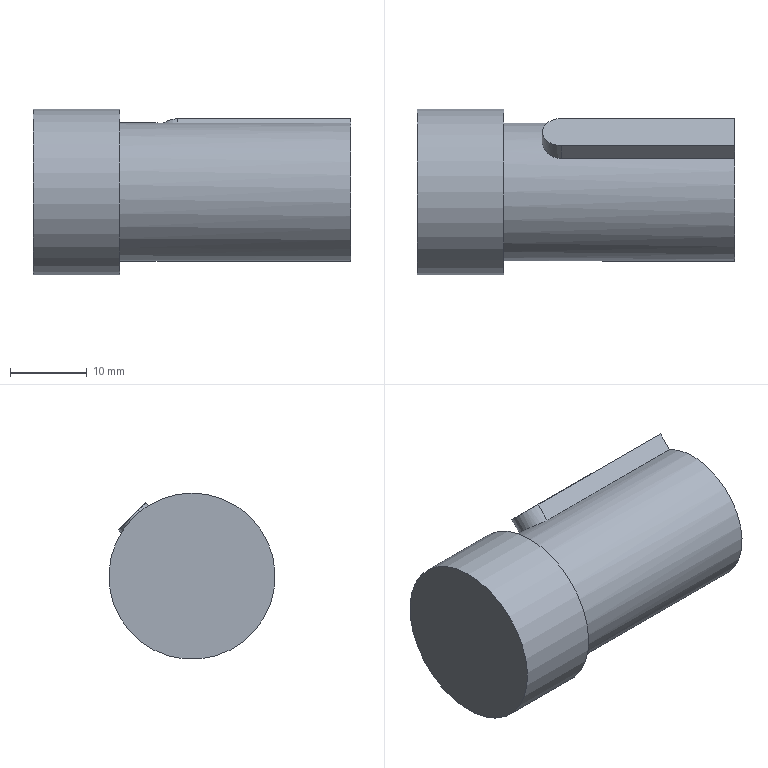Part | STEP file | basic_gh_motor_gh1_01 | 1 solid | 9 faces | box 41.25 x 21.6 x 21.6 mm | volume 12015 mm3 | plane 6 | cylinder 3 | commonest cylinder face diameters 5 x1 18 x1 21.6 x1
STEP:
#1=CARTESIAN_POINT('',(0.,92.846,7.881));
#2=VERTEX_POINT('',#1);
#3=CARTESIAN_POINT('',(-22.5,92.846,7.881));
#4=VERTEX_POINT('',#3);
#5=CARTESIAN_POINT('',(-11.25,92.846,7.881));
#6=DIRECTION('',(-1.,0.,0.));
#7=VECTOR('',#6,1.);
#8=LINE('',#5,#7);
#9=EDGE_CURVE('',#2,#4,#8,.T.);
#10=ORIENTED_EDGE('',*,*,#9,.F.);
#11=CARTESIAN_POINT('',(0.,94.51,9.546));
#12=VERTEX_POINT('',#11);
#13=CARTESIAN_POINT('',(0.,90.621,5.657));
#14=DIRECTION('',(0.,-0.7071,-0.7071));
#15=VECTOR('',#14,1.);
#16=LINE('',#13,#15);
#17=EDGE_CURVE('',#12,#2,#16,.T.);
#18=ORIENTED_EDGE('',*,*,#17,.F.);
#19=CARTESIAN_POINT('',(-22.5,94.51,9.546));
#20=VERTEX_POINT('',#19);
#21=CARTESIAN_POINT('',(-11.25,94.51,9.546));
#22=DIRECTION('',(1.,0.,0.));
#23=VECTOR('',#22,1.);
#24=LINE('',#21,#23);
#25=EDGE_CURVE('',#20,#12,#24,.T.);
#26=ORIENTED_EDGE('',*,*,#25,.F.);
#27=CARTESIAN_POINT('',(-22.5,90.621,5.657));
#28=DIRECTION('',(0.,-0.7071,-0.7071));
#29=VECTOR('',#28,1.);
#30=LINE('',#27,#29);
#31=EDGE_CURVE('',#20,#4,#30,.T.);
#32=ORIENTED_EDGE('',*,*,#31,.T.);
#33=EDGE_LOOP('',(#10,#18,#26,#32));
#34=FACE_OUTER_BOUND('',#33,.T.);
#35=CARTESIAN_POINT('',(-11.25,90.621,5.657));
#36=DIRECTION('',(0.,0.7071,-0.7071));
#37=DIRECTION('',(0.,0.7071,0.7071));
#38=AXIS2_PLACEMENT_3D('',#35,#36,#37);
#39=PLANE('',#38);
#40=ADVANCED_FACE('',(#34),#39,.F.);
#41=CARTESIAN_POINT('',(-22.5,96.381,4.346));
#42=VERTEX_POINT('',#41);
#43=CARTESIAN_POINT('',(-22.5,92.846,7.881));
#44=CARTESIAN_POINT('',(-22.658,92.846,7.881));
#45=CARTESIAN_POINT('',(-22.821,92.86,7.874));
#46=CARTESIAN_POINT('',(-23.144,92.917,7.841));
#47=CARTESIAN_POINT('',(-23.305,92.961,7.817));
#48=CARTESIAN_POINT('',(-23.613,93.076,7.75));
#49=CARTESIAN_POINT('',(-23.76,93.146,7.709));
#50=CARTESIAN_POINT('',(-24.032,93.306,7.61));
#51=CARTESIAN_POINT('',(-24.157,93.396,7.552));
#52=CARTESIAN_POINT('',(-24.378,93.584,7.428));
#53=CARTESIAN_POINT('',(-24.482,93.688,7.355));
#54=CARTESIAN_POINT('',(-24.665,93.911,7.193));
#55=CARTESIAN_POINT('',(-24.745,94.029,7.103));
#56=CARTESIAN_POINT('',(-24.873,94.27,6.909));
#57=CARTESIAN_POINT('',(-24.921,94.393,6.804));
#58=CARTESIAN_POINT('',(-24.985,94.634,6.588));
#59=CARTESIAN_POINT('',(-25.,94.752,6.476));
#60=CARTESIAN_POINT('',(-25.,94.976,6.252));
#61=CARTESIAN_POINT('',(-24.985,95.088,6.134));
#62=CARTESIAN_POINT('',(-24.921,95.304,5.893));
#63=CARTESIAN_POINT('',(-24.873,95.409,5.77));
#64=CARTESIAN_POINT('',(-24.745,95.603,5.529));
#65=CARTESIAN_POINT('',(-24.665,95.693,5.411));
#66=CARTESIAN_POINT('',(-24.482,95.855,5.188));
#67=CARTESIAN_POINT('',(-24.378,95.928,5.084));
#68=CARTESIAN_POINT('',(-24.157,96.052,4.896));
#69=CARTESIAN_POINT('',(-24.032,96.11,4.806));
#70=CARTESIAN_POINT('',(-23.76,96.209,4.646));
#71=CARTESIAN_POINT('',(-23.613,96.25,4.576));
#72=CARTESIAN_POINT('',(-23.305,96.317,4.461));
#73=CARTESIAN_POINT('',(-23.144,96.341,4.417));
#74=CARTESIAN_POINT('',(-22.821,96.374,4.36));
#75=CARTESIAN_POINT('',(-22.658,96.381,4.346));
#76=CARTESIAN_POINT('',(-22.5,96.381,4.346));
#77=B_SPLINE_CURVE_WITH_KNOTS('',3,(#43,#44,#45,#46,#47,#48,#49,#50,#51,#52,#53,#54,#55,#56,#57,#58,#59,#60,#61,#62,#63,#64,#65,#66,#67,#68,#69,#70,#71,#72,#73,#74,#75,#76),.UNSPECIFIED.,.F.,.F.,(4,2,2,2,2,2,2,2,2,2,2,2,2,2,2,2,4),(-7.577,-7.103,-6.63,-6.156,-5.682,-5.209,-4.735,-4.262,-3.788,-3.315,-2.841,-2.368,-1.894,-1.421,-0.9472,-0.4736,0.),.UNSPECIFIED.);
#78=EDGE_CURVE('',#4,#42,#77,.T.);
#79=ORIENTED_EDGE('',*,*,#78,.F.);
#80=ORIENTED_EDGE('',*,*,#31,.F.);
#81=CARTESIAN_POINT('',(-22.5,98.046,6.01));
#82=VERTEX_POINT('',#81);
#83=CARTESIAN_POINT('',(-22.5,96.278,7.778));
#84=DIRECTION('',(0.,0.7071,0.7071));
#85=DIRECTION('',(1.,0.,0.));
#86=AXIS2_PLACEMENT_3D('',#83,#84,#85);
#87=CIRCLE('',#86,2.5);
#88=EDGE_CURVE('',#82,#20,#87,.T.);
#89=ORIENTED_EDGE('',*,*,#88,.F.);
#90=CARTESIAN_POINT('',(-22.5,94.157,2.121));
#91=DIRECTION('',(0.,-0.7071,-0.7071));
#92=VECTOR('',#91,1.);
#93=LINE('',#90,#92);
#94=EDGE_CURVE('',#82,#42,#93,.T.);
#95=ORIENTED_EDGE('',*,*,#94,.T.);
#96=EDGE_LOOP('',(#79,#80,#89,#95));
#97=FACE_OUTER_BOUND('',#96,.T.);
#98=CARTESIAN_POINT('',(-22.5,92.389,3.889));
#99=DIRECTION('',(0.,0.7071,0.7071));
#100=DIRECTION('',(-1.,0.,0.));
#101=AXIS2_PLACEMENT_3D('',#98,#99,#100);
#102=CYLINDRICAL_SURFACE('',#101,2.5);
#103=ADVANCED_FACE('',(#97),#102,.T.);
#104=CARTESIAN_POINT('',(0.,98.046,6.01));
#105=VERTEX_POINT('',#104);
#106=CARTESIAN_POINT('',(-11.25,98.046,6.01));
#107=DIRECTION('',(-1.,0.,0.));
#108=VECTOR('',#107,1.);
#109=LINE('',#106,#108);
#110=EDGE_CURVE('',#105,#82,#109,.T.);
#111=ORIENTED_EDGE('',*,*,#110,.T.);
#112=ORIENTED_EDGE('',*,*,#88,.T.);
#113=ORIENTED_EDGE('',*,*,#25,.T.);
#114=CARTESIAN_POINT('',(0.,96.278,7.778));
#115=DIRECTION('',(0.,0.7071,-0.7071));
#116=VECTOR('',#115,1.);
#117=LINE('',#114,#116);
#118=EDGE_CURVE('',#12,#105,#117,.T.);
#119=ORIENTED_EDGE('',*,*,#118,.T.);
#120=EDGE_LOOP('',(#111,#112,#113,#119));
#121=FACE_OUTER_BOUND('',#120,.T.);
#122=CARTESIAN_POINT('',(-11.25,96.278,7.778));
#123=DIRECTION('',(0.,0.7071,0.7071));
#124=DIRECTION('',(1.,0.,0.));
#125=AXIS2_PLACEMENT_3D('',#122,#123,#124);
#126=PLANE('',#125);
#127=ADVANCED_FACE('',(#121),#126,.T.);
#128=CARTESIAN_POINT('',(0.,96.381,4.346));
#129=VERTEX_POINT('',#128);
#130=CARTESIAN_POINT('',(-11.25,96.381,4.346));
#131=DIRECTION('',(1.,0.,0.));
#132=VECTOR('',#131,1.);
#133=LINE('',#130,#132);
#134=EDGE_CURVE('',#42,#129,#133,.T.);
#135=ORIENTED_EDGE('',*,*,#134,.F.);
#136=ORIENTED_EDGE('',*,*,#94,.F.);
#137=ORIENTED_EDGE('',*,*,#110,.F.);
#138=CARTESIAN_POINT('',(0.,94.157,2.121));
#139=DIRECTION('',(0.,-0.7071,-0.7071));
#140=VECTOR('',#139,1.);
#141=LINE('',#138,#140);
#142=EDGE_CURVE('',#105,#129,#141,.T.);
#143=ORIENTED_EDGE('',*,*,#142,.T.);
#144=EDGE_LOOP('',(#135,#136,#137,#143));
#145=FACE_OUTER_BOUND('',#144,.T.);
#146=CARTESIAN_POINT('',(-11.25,94.157,2.121));
#147=DIRECTION('',(0.,-0.7071,0.7071));
#148=DIRECTION('',(0.,-0.7071,-0.7071));
#149=AXIS2_PLACEMENT_3D('',#146,#147,#148);
#150=PLANE('',#149);
#151=ADVANCED_FACE('',(#145),#150,.F.);
#152=CARTESIAN_POINT('',(-30.,88.5,-9.));
#153=VERTEX_POINT('',#152);
#154=CARTESIAN_POINT('',(-30.,88.5,0.));
#155=DIRECTION('',(-1.,0.,0.));
#156=DIRECTION('',(0.,0.,1.));
#157=AXIS2_PLACEMENT_3D('',#154,#155,#156);
#158=CIRCLE('',#157,9.);
#159=EDGE_CURVE('',#153,#153,#158,.T.);
#160=ORIENTED_EDGE('',*,*,#159,.F.);
#161=CARTESIAN_POINT('',(0.,88.5,-9.));
#162=VERTEX_POINT('',#161);
#163=CARTESIAN_POINT('',(-15.05,88.5,-9.));
#164=DIRECTION('',(1.,0.,0.));
#165=VECTOR('',#164,9.);
#166=LINE('',#163,#165);
#167=EDGE_CURVE('',#153,#162,#166,.T.);
#168=ORIENTED_EDGE('',*,*,#167,.T.);
#169=CARTESIAN_POINT('',(0.,88.5,0.));
#170=DIRECTION('',(1.,0.,0.));
#171=DIRECTION('',(0.,0.,1.));
#172=AXIS2_PLACEMENT_3D('',#169,#170,#171);
#173=CIRCLE('',#172,9.);
#174=EDGE_CURVE('',#2,#162,#173,.T.);
#175=ORIENTED_EDGE('',*,*,#174,.F.);
#176=ORIENTED_EDGE('',*,*,#9,.T.);
#177=ORIENTED_EDGE('',*,*,#78,.T.);
#178=ORIENTED_EDGE('',*,*,#134,.T.);
#179=CARTESIAN_POINT('',(0.,88.5,0.));
#180=DIRECTION('',(1.,0.,0.));
#181=DIRECTION('',(0.,0.,1.));
#182=AXIS2_PLACEMENT_3D('',#179,#180,#181);
#183=CIRCLE('',#182,9.);
#184=EDGE_CURVE('',#162,#129,#183,.T.);
#185=ORIENTED_EDGE('',*,*,#184,.F.);
#186=ORIENTED_EDGE('',*,*,#167,.F.);
#187=EDGE_LOOP('',(#160,#168,#175,#176,#177,#178,#185,#186));
#188=FACE_OUTER_BOUND('',#187,.T.);
#189=CARTESIAN_POINT('',(-15.05,88.5,0.));
#190=DIRECTION('',(-1.,0.,0.));
#191=DIRECTION('',(0.,0.,1.));
#192=AXIS2_PLACEMENT_3D('',#189,#190,#191);
#193=CYLINDRICAL_SURFACE('',#192,9.);
#194=ADVANCED_FACE('',(#188),#193,.T.);
#195=ORIENTED_EDGE('',*,*,#174,.T.);
#196=ORIENTED_EDGE('',*,*,#184,.T.);
#197=ORIENTED_EDGE('',*,*,#142,.F.);
#198=ORIENTED_EDGE('',*,*,#118,.F.);
#199=ORIENTED_EDGE('',*,*,#17,.T.);
#200=EDGE_LOOP('',(#195,#196,#197,#198,#199));
#201=FACE_OUTER_BOUND('',#200,.T.);
#202=CARTESIAN_POINT('',(0.,88.5,0.));
#203=DIRECTION('',(1.,0.,0.));
#204=DIRECTION('',(0.,0.,-1.));
#205=AXIS2_PLACEMENT_3D('',#202,#203,#204);
#206=PLANE('',#205);
#207=ADVANCED_FACE('',(#201),#206,.T.);
#208=CARTESIAN_POINT('',(-30.,88.5,10.8));
#209=VERTEX_POINT('',#208);
#210=CARTESIAN_POINT('',(-30.,88.5,0.));
#211=DIRECTION('',(1.,0.,0.));
#212=DIRECTION('',(0.,0.,-1.));
#213=AXIS2_PLACEMENT_3D('',#210,#211,#212);
#214=CIRCLE('',#213,10.8);
#215=EDGE_CURVE('',#209,#209,#214,.T.);
#216=ORIENTED_EDGE('',*,*,#215,.F.);
#217=CARTESIAN_POINT('',(-41.25,88.5,10.8));
#218=VERTEX_POINT('',#217);
#219=CARTESIAN_POINT('',(-35.625,88.5,10.8));
#220=DIRECTION('',(-1.,0.,0.));
#221=VECTOR('',#220,10.8);
#222=LINE('',#219,#221);
#223=EDGE_CURVE('',#209,#218,#222,.T.);
#224=ORIENTED_EDGE('',*,*,#223,.T.);
#225=CARTESIAN_POINT('',(-41.25,88.5,0.));
#226=DIRECTION('',(-1.,0.,0.));
#227=DIRECTION('',(0.,0.,-1.));
#228=AXIS2_PLACEMENT_3D('',#225,#226,#227);
#229=CIRCLE('',#228,10.8);
#230=EDGE_CURVE('',#218,#218,#229,.T.);
#231=ORIENTED_EDGE('',*,*,#230,.F.);
#232=ORIENTED_EDGE('',*,*,#223,.F.);
#233=EDGE_LOOP('',(#216,#224,#231,#232));
#234=FACE_OUTER_BOUND('',#233,.T.);
#235=CARTESIAN_POINT('',(-35.625,88.5,0.));
#236=DIRECTION('',(1.,0.,0.));
#237=DIRECTION('',(0.,0.,-1.));
#238=AXIS2_PLACEMENT_3D('',#235,#236,#237);
#239=CYLINDRICAL_SURFACE('',#238,10.8);
#240=ADVANCED_FACE('',(#234),#239,.T.);
#241=ORIENTED_EDGE('',*,*,#230,.T.);
#242=EDGE_LOOP('',(#241));
#243=FACE_OUTER_BOUND('',#242,.T.);
#244=CARTESIAN_POINT('',(-41.25,88.5,0.));
#245=DIRECTION('',(-1.,0.,0.));
#246=DIRECTION('',(0.,0.,1.));
#247=AXIS2_PLACEMENT_3D('',#244,#245,#246);
#248=PLANE('',#247);
#249=ADVANCED_FACE('',(#243),#248,.T.);
#250=ORIENTED_EDGE('',*,*,#215,.T.);
#251=EDGE_LOOP('',(#250));
#252=FACE_OUTER_BOUND('',#251,.T.);
#253=ORIENTED_EDGE('',*,*,#159,.T.);
#254=EDGE_LOOP('',(#253));
#255=FACE_BOUND('',#254,.T.);
#256=CARTESIAN_POINT('',(-30.,88.5,0.));
#257=DIRECTION('',(1.,0.,0.));
#258=DIRECTION('',(0.,0.,-1.));
#259=AXIS2_PLACEMENT_3D('',#256,#257,#258);
#260=PLANE('',#259);
#261=ADVANCED_FACE('',(#252,#255),#260,.T.);
#262=CLOSED_SHELL('',(#40,#103,#127,#151,#194,#207,#240,#249,#261));
#263=MANIFOLD_SOLID_BREP('',#262);
#264=(LENGTH_UNIT()NAMED_UNIT(*)SI_UNIT(.MILLI.,.METRE.));
#265=UNCERTAINTY_MEASURE_WITH_UNIT(LENGTH_MEASURE(0.01),#264,'','');
#266=(NAMED_UNIT(*)PLANE_ANGLE_UNIT()SI_UNIT($,.RADIAN.));
#267=(NAMED_UNIT(*)SI_UNIT($,.STERADIAN.)SOLID_ANGLE_UNIT());
#268=(GEOMETRIC_REPRESENTATION_CONTEXT(3)GLOBAL_UNCERTAINTY_ASSIGNED_CONTEXT((#265))GLOBAL_UNIT_ASSIGNED_CONTEXT((#264,#266,#267))REPRESENTATION_CONTEXT('',''));
#269=ADVANCED_BREP_SHAPE_REPRESENTATION('',(#263),#268);